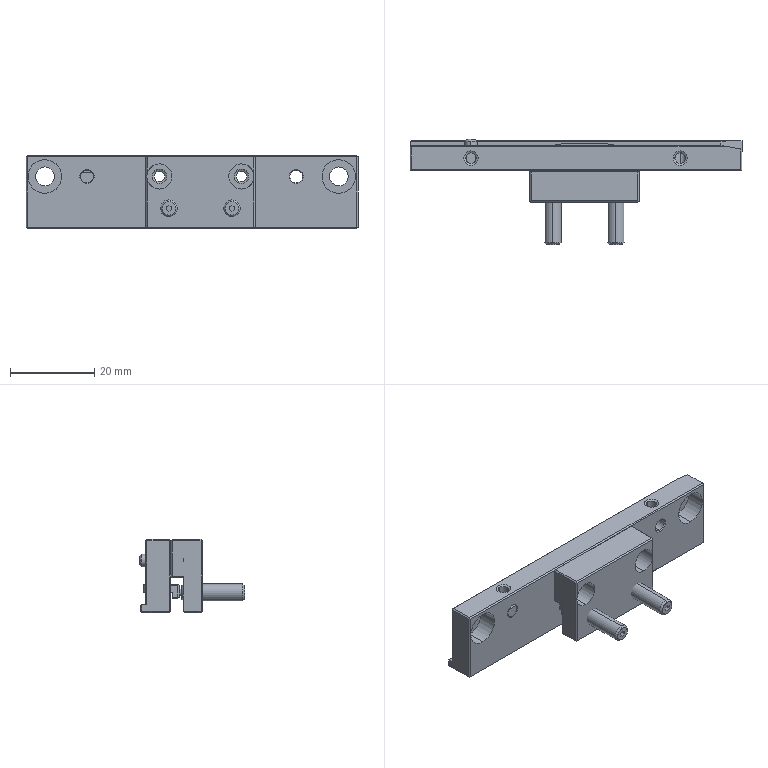Part | NX | 7 solids | 186 faces | box 79 x 25.105 x 17.4 mm | volume 10789 mm3 | plane 105 | cylinder 52 | cone 26 | sphere 3 | commonest cylinder face diameters 2.5 x8 1.6 x6 3 x6 3.2 x6 4 x6 3.3 x4